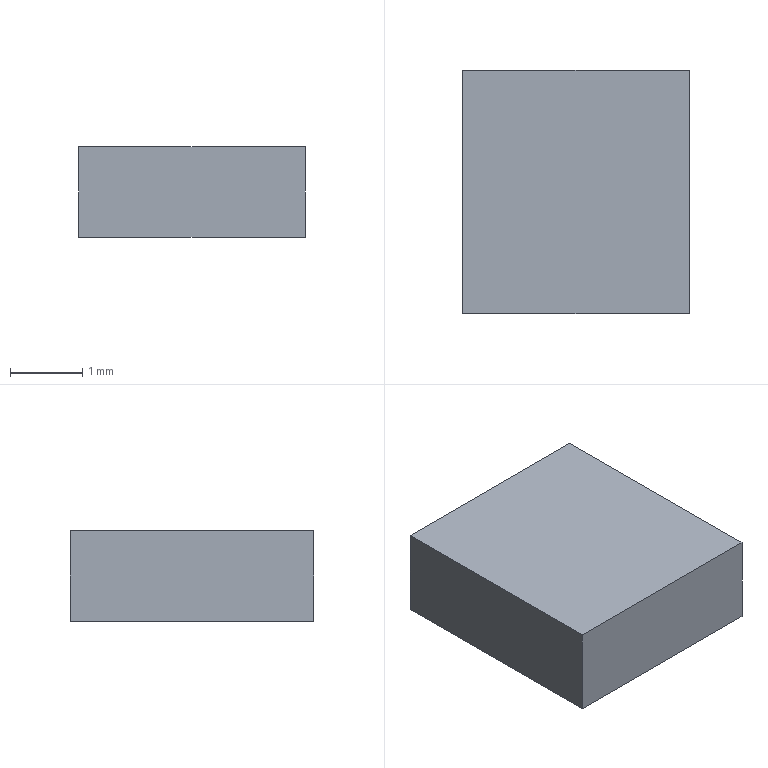Part | Creo | 1 solid | 6 faces | box 3.127 x 3.363 x 1.25 mm | volume 13.145 mm3 | plane 6
STEP:
#1=CARTESIAN_POINT('',(0.,0.,0.));
#2=DIRECTION('',(0.,0.,1.));
#3=DIRECTION('',(1.,0.,0.));
#4=AXIS2_PLACEMENT_3D('',#1,#2,#3);
#5=CARTESIAN_POINT('',(-1.575,-2.863,0.));
#6=VERTEX_POINT('',#5);
#7=CARTESIAN_POINT('',(1.552,-2.863,0.));
#8=VERTEX_POINT('',#7);
#9=CARTESIAN_POINT('',(-1.575,-2.863,0.));
#10=DIRECTION('',(1.,0.,0.));
#11=VECTOR('',#10,3.127);
#12=LINE('',#9,#11);
#13=EDGE_CURVE('',#6,#8,#12,.T.);
#14=ORIENTED_EDGE('',*,*,#13,.T.);
#15=CARTESIAN_POINT('',(1.552,0.5004,0.));
#16=VERTEX_POINT('',#15);
#17=CARTESIAN_POINT('',(1.552,-2.863,0.));
#18=DIRECTION('',(0.,1.,0.));
#19=VECTOR('',#18,3.363);
#20=LINE('',#17,#19);
#21=EDGE_CURVE('',#8,#16,#20,.T.);
#22=ORIENTED_EDGE('',*,*,#21,.T.);
#23=CARTESIAN_POINT('',(-1.575,0.5004,0.));
#24=VERTEX_POINT('',#23);
#25=CARTESIAN_POINT('',(1.552,0.5004,0.));
#26=DIRECTION('',(-1.,0.,0.));
#27=VECTOR('',#26,3.127);
#28=LINE('',#25,#27);
#29=EDGE_CURVE('',#16,#24,#28,.T.);
#30=ORIENTED_EDGE('',*,*,#29,.T.);
#31=CARTESIAN_POINT('',(-1.575,0.5004,0.));
#32=DIRECTION('',(0.,-1.,0.));
#33=VECTOR('',#32,3.363);
#34=LINE('',#31,#33);
#35=EDGE_CURVE('',#24,#6,#34,.T.);
#36=ORIENTED_EDGE('',*,*,#35,.T.);
#37=EDGE_LOOP('',(#14,#22,#30,#36));
#38=FACE_OUTER_BOUND('',#37,.F.);
#39=CARTESIAN_POINT('',(0.,0.,0.));
#40=DIRECTION('',(0.,0.,1.));
#41=DIRECTION('',(1.,0.,0.));
#42=AXIS2_PLACEMENT_3D('',#39,#40,#41);
#43=PLANE('',#42);
#44=ADVANCED_FACE('',(#38),#43,.F.);
#45=ORIENTED_EDGE('',*,*,#13,.F.);
#46=CARTESIAN_POINT('',(-1.575,-2.863,1.25));
#47=VERTEX_POINT('',#46);
#48=CARTESIAN_POINT('',(-1.575,-2.863,0.));
#49=DIRECTION('',(0.,0.,1.));
#50=VECTOR('',#49,1.25);
#51=LINE('',#48,#50);
#52=EDGE_CURVE('',#6,#47,#51,.T.);
#53=ORIENTED_EDGE('',*,*,#52,.T.);
#54=CARTESIAN_POINT('',(1.552,-2.863,1.25));
#55=VERTEX_POINT('',#54);
#56=CARTESIAN_POINT('',(-1.575,-2.863,1.25));
#57=DIRECTION('',(1.,0.,0.));
#58=VECTOR('',#57,3.127);
#59=LINE('',#56,#58);
#60=EDGE_CURVE('',#47,#55,#59,.T.);
#61=ORIENTED_EDGE('',*,*,#60,.T.);
#62=CARTESIAN_POINT('',(1.552,-2.863,0.));
#63=DIRECTION('',(0.,0.,1.));
#64=VECTOR('',#63,1.25);
#65=LINE('',#62,#64);
#66=EDGE_CURVE('',#8,#55,#65,.T.);
#67=ORIENTED_EDGE('',*,*,#66,.F.);
#68=EDGE_LOOP('',(#45,#53,#61,#67));
#69=FACE_OUTER_BOUND('',#68,.F.);
#70=CARTESIAN_POINT('',(-1.575,-2.863,0.));
#71=DIRECTION('',(0.,-1.,0.));
#72=DIRECTION('',(1.,0.,0.));
#73=AXIS2_PLACEMENT_3D('',#70,#71,#72);
#74=PLANE('',#73);
#75=ADVANCED_FACE('',(#69),#74,.T.);
#76=ORIENTED_EDGE('',*,*,#35,.F.);
#77=CARTESIAN_POINT('',(-1.575,0.5004,1.25));
#78=VERTEX_POINT('',#77);
#79=CARTESIAN_POINT('',(-1.575,0.5004,0.));
#80=DIRECTION('',(0.,0.,1.));
#81=VECTOR('',#80,1.25);
#82=LINE('',#79,#81);
#83=EDGE_CURVE('',#24,#78,#82,.T.);
#84=ORIENTED_EDGE('',*,*,#83,.T.);
#85=CARTESIAN_POINT('',(-1.575,0.5004,1.25));
#86=DIRECTION('',(0.,-1.,0.));
#87=VECTOR('',#86,3.363);
#88=LINE('',#85,#87);
#89=EDGE_CURVE('',#78,#47,#88,.T.);
#90=ORIENTED_EDGE('',*,*,#89,.T.);
#91=ORIENTED_EDGE('',*,*,#52,.F.);
#92=EDGE_LOOP('',(#76,#84,#90,#91));
#93=FACE_OUTER_BOUND('',#92,.F.);
#94=CARTESIAN_POINT('',(-1.575,0.5004,0.));
#95=DIRECTION('',(-1.,0.,0.));
#96=DIRECTION('',(0.,-1.,0.));
#97=AXIS2_PLACEMENT_3D('',#94,#95,#96);
#98=PLANE('',#97);
#99=ADVANCED_FACE('',(#93),#98,.T.);
#100=ORIENTED_EDGE('',*,*,#29,.F.);
#101=CARTESIAN_POINT('',(1.552,0.5004,1.25));
#102=VERTEX_POINT('',#101);
#103=CARTESIAN_POINT('',(1.552,0.5004,0.));
#104=DIRECTION('',(0.,0.,1.));
#105=VECTOR('',#104,1.25);
#106=LINE('',#103,#105);
#107=EDGE_CURVE('',#16,#102,#106,.T.);
#108=ORIENTED_EDGE('',*,*,#107,.T.);
#109=CARTESIAN_POINT('',(1.552,0.5004,1.25));
#110=DIRECTION('',(-1.,0.,0.));
#111=VECTOR('',#110,3.127);
#112=LINE('',#109,#111);
#113=EDGE_CURVE('',#102,#78,#112,.T.);
#114=ORIENTED_EDGE('',*,*,#113,.T.);
#115=ORIENTED_EDGE('',*,*,#83,.F.);
#116=EDGE_LOOP('',(#100,#108,#114,#115));
#117=FACE_OUTER_BOUND('',#116,.F.);
#118=CARTESIAN_POINT('',(1.552,0.5004,0.));
#119=DIRECTION('',(0.,1.,0.));
#120=DIRECTION('',(-1.,0.,0.));
#121=AXIS2_PLACEMENT_3D('',#118,#119,#120);
#122=PLANE('',#121);
#123=ADVANCED_FACE('',(#117),#122,.T.);
#124=ORIENTED_EDGE('',*,*,#21,.F.);
#125=ORIENTED_EDGE('',*,*,#66,.T.);
#126=CARTESIAN_POINT('',(1.552,-2.863,1.25));
#127=DIRECTION('',(0.,1.,0.));
#128=VECTOR('',#127,3.363);
#129=LINE('',#126,#128);
#130=EDGE_CURVE('',#55,#102,#129,.T.);
#131=ORIENTED_EDGE('',*,*,#130,.T.);
#132=ORIENTED_EDGE('',*,*,#107,.F.);
#133=EDGE_LOOP('',(#124,#125,#131,#132));
#134=FACE_OUTER_BOUND('',#133,.F.);
#135=CARTESIAN_POINT('',(1.552,-2.863,0.));
#136=DIRECTION('',(1.,0.,0.));
#137=DIRECTION('',(0.,1.,0.));
#138=AXIS2_PLACEMENT_3D('',#135,#136,#137);
#139=PLANE('',#138);
#140=ADVANCED_FACE('',(#134),#139,.T.);
#141=ORIENTED_EDGE('',*,*,#60,.F.);
#142=ORIENTED_EDGE('',*,*,#89,.F.);
#143=ORIENTED_EDGE('',*,*,#113,.F.);
#144=ORIENTED_EDGE('',*,*,#130,.F.);
#145=EDGE_LOOP('',(#141,#142,#143,#144));
#146=FACE_OUTER_BOUND('',#145,.F.);
#147=CARTESIAN_POINT('',(0.,0.,1.25));
#148=DIRECTION('',(0.,0.,1.));
#149=DIRECTION('',(1.,0.,0.));
#150=AXIS2_PLACEMENT_3D('',#147,#148,#149);
#151=PLANE('',#150);
#152=ADVANCED_FACE('',(#146),#151,.T.);
#153=CLOSED_SHELL('',(#44,#75,#99,#123,#140,#152));
#154=MANIFOLD_SOLID_BREP('',#153);
#155=(LENGTH_UNIT()NAMED_UNIT(*)SI_UNIT(.MILLI.,.METRE.));
#156=UNCERTAINTY_MEASURE_WITH_UNIT(LENGTH_MEASURE(0.0004759),#155,'','');
#157=(NAMED_UNIT(*)PLANE_ANGLE_UNIT()SI_UNIT($,.RADIAN.));
#158=PLANE_ANGLE_MEASURE_WITH_UNIT(PLANE_ANGLE_MEASURE(0.01745),#157);
#159=(CONVERSION_BASED_UNIT('DEGREE',#158)NAMED_UNIT(*)PLANE_ANGLE_UNIT());
#160=(NAMED_UNIT(*)SI_UNIT($,.STERADIAN.)SOLID_ANGLE_UNIT());
#161=(GEOMETRIC_REPRESENTATION_CONTEXT(3)GLOBAL_UNCERTAINTY_ASSIGNED_CONTEXT((#156))GLOBAL_UNIT_ASSIGNED_CONTEXT((#155,#159,#160))REPRESENTATION_CONTEXT('',''));
#162=ADVANCED_BREP_SHAPE_REPRESENTATION('',(#4,#154),#161);